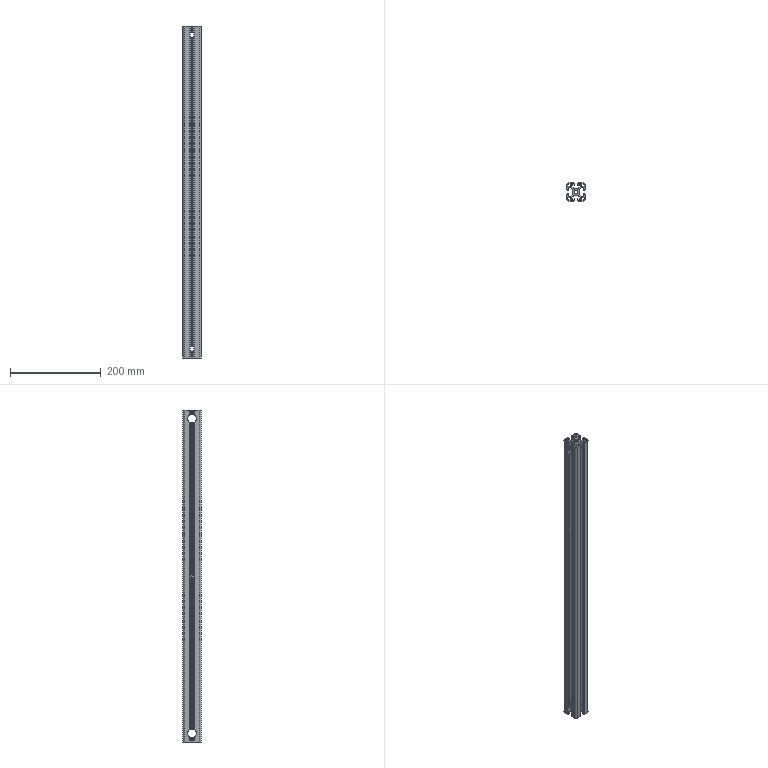Part | SolidWorks | features Extrusion 1, HoleWzd 1 | 1 solid | 273 faces | box 40 x 40 x 730 mm | volume 430419 mm3 | plane 213 | cylinder 60 | commonest cylinder face diameters 2 x16 6.8 x15 19 x12 1 x8 5 x4 9 x4